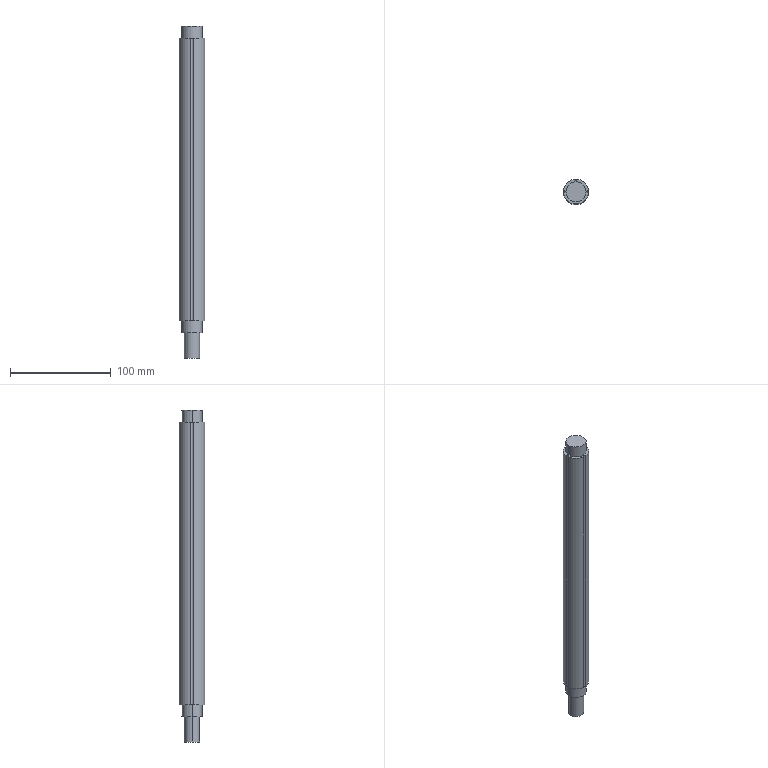Part | SolidWorks | features ICE 4, CirPattern 1, Extrusion 1 | 1 solid | 20 faces | box 24.846 x 24.846 x 329 mm | volume 147174 mm3 | cylinder 15 | plane 5 | commonest cylinder face diameters 3 x5 20 x4 25 x4 15 x2
STEP:
#1=CARTESIAN_POINT('',(11.5,0.,280.));
#2=VERTEX_POINT('',#1);
#3=CARTESIAN_POINT('',(12.423,1.385,280.));
#4=VERTEX_POINT('',#3);
#5=CARTESIAN_POINT('',(13.,0.,280.));
#6=DIRECTION('',(0.,0.,-1.));
#7=DIRECTION('',(1.,0.,0.));
#8=AXIS2_PLACEMENT_3D('',#5,#6,#7);
#9=CIRCLE('',#8,1.5);
#10=EDGE_CURVE('',#2,#4,#9,.T.);
#11=ORIENTED_EDGE('',*,*,#10,.F.);
#12=CARTESIAN_POINT('',(11.5,0.,0.));
#13=VERTEX_POINT('',#12);
#14=CARTESIAN_POINT('',(11.5,0.,284.243));
#15=DIRECTION('',(0.,0.,-1.));
#16=VECTOR('',#15,1000.);
#17=LINE('',#14,#16);
#18=EDGE_CURVE('',#2,#13,#17,.T.);
#19=ORIENTED_EDGE('',*,*,#18,.T.);
#20=CARTESIAN_POINT('',(12.423,1.385,0.));
#21=VERTEX_POINT('',#20);
#22=CARTESIAN_POINT('',(13.,0.,0.));
#23=DIRECTION('',(0.,0.,-1.));
#24=DIRECTION('',(0.,1.,0.));
#25=AXIS2_PLACEMENT_3D('',#22,#23,#24);
#26=CIRCLE('',#25,1.5);
#27=EDGE_CURVE('',#13,#21,#26,.T.);
#28=ORIENTED_EDGE('',*,*,#27,.T.);
#29=CARTESIAN_POINT('',(12.423,1.385,140.));
#30=DIRECTION('',(0.,0.,-1.));
#31=VECTOR('',#30,1000.);
#32=LINE('',#29,#31);
#33=EDGE_CURVE('',#4,#21,#32,.T.);
#34=ORIENTED_EDGE('',*,*,#33,.F.);
#35=EDGE_LOOP('',(#11,#19,#28,#34));
#36=FACE_OUTER_BOUND('',#35,.T.);
#37=CARTESIAN_POINT('',(13.,0.,284.243));
#38=DIRECTION('',(0.,0.,-1.));
#39=DIRECTION('',(-1.,0.,0.));
#40=AXIS2_PLACEMENT_3D('',#37,#38,#39);
#41=CYLINDRICAL_SURFACE('',#40,1.5);
#42=ADVANCED_FACE('',(#36),#41,.F.);
#43=CARTESIAN_POINT('',(-7.5,0.,-37.));
#44=VERTEX_POINT('',#43);
#45=CARTESIAN_POINT('',(7.5,0.,-37.));
#46=VERTEX_POINT('',#45);
#47=CARTESIAN_POINT('',(0.,0.,-37.));
#48=DIRECTION('',(0.,0.,-1.));
#49=DIRECTION('',(-1.,0.,0.));
#50=AXIS2_PLACEMENT_3D('',#47,#48,#49);
#51=CIRCLE('',#50,7.5);
#52=EDGE_CURVE('',#44,#46,#51,.T.);
#53=ORIENTED_EDGE('',*,*,#52,.F.);
#54=CARTESIAN_POINT('',(-7.5,0.,-12.));
#55=VERTEX_POINT('',#54);
#56=CARTESIAN_POINT('',(-7.5,0.,-37.));
#57=DIRECTION('',(0.,0.,1.));
#58=VECTOR('',#57,1000.);
#59=LINE('',#56,#58);
#60=EDGE_CURVE('',#44,#55,#59,.T.);
#61=ORIENTED_EDGE('',*,*,#60,.T.);
#62=CARTESIAN_POINT('',(7.5,0.,-12.));
#63=VERTEX_POINT('',#62);
#64=CARTESIAN_POINT('',(0.,0.,-12.));
#65=DIRECTION('',(0.,0.,-1.));
#66=DIRECTION('',(-1.,0.,0.));
#67=AXIS2_PLACEMENT_3D('',#64,#65,#66);
#68=CIRCLE('',#67,7.5);
#69=EDGE_CURVE('',#55,#63,#68,.T.);
#70=ORIENTED_EDGE('',*,*,#69,.T.);
#71=CARTESIAN_POINT('',(7.5,0.,-37.));
#72=DIRECTION('',(0.,0.,1.));
#73=VECTOR('',#72,1000.);
#74=LINE('',#71,#73);
#75=EDGE_CURVE('',#46,#63,#74,.T.);
#76=ORIENTED_EDGE('',*,*,#75,.F.);
#77=EDGE_LOOP('',(#53,#61,#70,#76));
#78=FACE_OUTER_BOUND('',#77,.T.);
#79=CARTESIAN_POINT('',(0.,0.,-37.));
#80=DIRECTION('',(0.,0.,1.));
#81=DIRECTION('',(1.,0.,0.));
#82=AXIS2_PLACEMENT_3D('',#79,#80,#81);
#83=CYLINDRICAL_SURFACE('',#82,7.5);
#84=ADVANCED_FACE('',(#78),#83,.T.);
#85=CARTESIAN_POINT('',(-10.,0.,-12.));
#86=VERTEX_POINT('',#85);
#87=CARTESIAN_POINT('',(10.,0.,-12.));
#88=VERTEX_POINT('',#87);
#89=CARTESIAN_POINT('',(0.,0.,-12.));
#90=DIRECTION('',(0.,0.,-1.));
#91=DIRECTION('',(-1.,0.,0.));
#92=AXIS2_PLACEMENT_3D('',#89,#90,#91);
#93=CIRCLE('',#92,10.);
#94=EDGE_CURVE('',#86,#88,#93,.T.);
#95=ORIENTED_EDGE('',*,*,#94,.F.);
#96=CARTESIAN_POINT('',(-10.,0.,0.));
#97=VERTEX_POINT('',#96);
#98=CARTESIAN_POINT('',(-10.,0.,-12.));
#99=DIRECTION('',(0.,0.,1.));
#100=VECTOR('',#99,1000.);
#101=LINE('',#98,#100);
#102=EDGE_CURVE('',#86,#97,#101,.T.);
#103=ORIENTED_EDGE('',*,*,#102,.T.);
#104=CARTESIAN_POINT('',(10.,0.,0.));
#105=VERTEX_POINT('',#104);
#106=CARTESIAN_POINT('',(0.,0.,0.));
#107=DIRECTION('',(0.,0.,-1.));
#108=DIRECTION('',(-1.,0.,0.));
#109=AXIS2_PLACEMENT_3D('',#106,#107,#108);
#110=CIRCLE('',#109,10.);
#111=EDGE_CURVE('',#97,#105,#110,.T.);
#112=ORIENTED_EDGE('',*,*,#111,.T.);
#113=CARTESIAN_POINT('',(10.,0.,-12.));
#114=DIRECTION('',(0.,0.,1.));
#115=VECTOR('',#114,1000.);
#116=LINE('',#113,#115);
#117=EDGE_CURVE('',#88,#105,#116,.T.);
#118=ORIENTED_EDGE('',*,*,#117,.F.);
#119=EDGE_LOOP('',(#95,#103,#112,#118));
#120=FACE_OUTER_BOUND('',#119,.T.);
#121=CARTESIAN_POINT('',(0.,0.,-12.));
#122=DIRECTION('',(0.,0.,1.));
#123=DIRECTION('',(1.,0.,0.));
#124=AXIS2_PLACEMENT_3D('',#121,#122,#123);
#125=CYLINDRICAL_SURFACE('',#124,10.);
#126=ADVANCED_FACE('',(#120),#125,.T.);
#127=CARTESIAN_POINT('',(10.,0.,292.));
#128=VERTEX_POINT('',#127);
#129=CARTESIAN_POINT('',(-10.,0.,292.));
#130=VERTEX_POINT('',#129);
#131=CARTESIAN_POINT('',(0.,0.,292.));
#132=DIRECTION('',(0.,0.,1.));
#133=DIRECTION('',(1.,0.,0.));
#134=AXIS2_PLACEMENT_3D('',#131,#132,#133);
#135=CIRCLE('',#134,10.);
#136=EDGE_CURVE('',#128,#130,#135,.T.);
#137=ORIENTED_EDGE('',*,*,#136,.F.);
#138=CARTESIAN_POINT('',(10.,0.,280.));
#139=VERTEX_POINT('',#138);
#140=CARTESIAN_POINT('',(10.,0.,292.));
#141=DIRECTION('',(0.,0.,-1.));
#142=VECTOR('',#141,1000.);
#143=LINE('',#140,#142);
#144=EDGE_CURVE('',#128,#139,#143,.T.);
#145=ORIENTED_EDGE('',*,*,#144,.T.);
#146=CARTESIAN_POINT('',(-10.,0.,280.));
#147=VERTEX_POINT('',#146);
#148=CARTESIAN_POINT('',(0.,0.,280.));
#149=DIRECTION('',(0.,0.,1.));
#150=DIRECTION('',(1.,0.,0.));
#151=AXIS2_PLACEMENT_3D('',#148,#149,#150);
#152=CIRCLE('',#151,10.);
#153=EDGE_CURVE('',#139,#147,#152,.T.);
#154=ORIENTED_EDGE('',*,*,#153,.T.);
#155=CARTESIAN_POINT('',(-10.,0.,292.));
#156=DIRECTION('',(0.,0.,-1.));
#157=VECTOR('',#156,1000.);
#158=LINE('',#155,#157);
#159=EDGE_CURVE('',#130,#147,#158,.T.);
#160=ORIENTED_EDGE('',*,*,#159,.F.);
#161=EDGE_LOOP('',(#137,#145,#154,#160));
#162=FACE_OUTER_BOUND('',#161,.T.);
#163=CARTESIAN_POINT('',(0.,0.,292.));
#164=DIRECTION('',(0.,0.,-1.));
#165=DIRECTION('',(-1.,0.,0.));
#166=AXIS2_PLACEMENT_3D('',#163,#164,#165);
#167=CYLINDRICAL_SURFACE('',#166,10.);
#168=ADVANCED_FACE('',(#162),#167,.T.);
#169=CARTESIAN_POINT('',(1.385,-12.423,0.));
#170=VERTEX_POINT('',#169);
#171=CARTESIAN_POINT('',(12.423,-1.385,0.));
#172=VERTEX_POINT('',#171);
#173=CARTESIAN_POINT('',(0.,0.,0.));
#174=DIRECTION('',(0.,0.,1.));
#175=DIRECTION('',(1.,0.,0.));
#176=AXIS2_PLACEMENT_3D('',#173,#174,#175);
#177=CIRCLE('',#176,12.5);
#178=EDGE_CURVE('',#170,#172,#177,.T.);
#179=ORIENTED_EDGE('',*,*,#178,.T.);
#180=CARTESIAN_POINT('',(12.423,-1.385,280.));
#181=VERTEX_POINT('',#180);
#182=CARTESIAN_POINT('',(12.423,-1.385,140.));
#183=DIRECTION('',(0.,0.,1.));
#184=VECTOR('',#183,1000.);
#185=LINE('',#182,#184);
#186=EDGE_CURVE('',#172,#181,#185,.T.);
#187=ORIENTED_EDGE('',*,*,#186,.T.);
#188=CARTESIAN_POINT('',(1.385,-12.423,280.));
#189=VERTEX_POINT('',#188);
#190=CARTESIAN_POINT('',(0.,0.,280.));
#191=DIRECTION('',(0.,0.,1.));
#192=DIRECTION('',(1.,0.,0.));
#193=AXIS2_PLACEMENT_3D('',#190,#191,#192);
#194=CIRCLE('',#193,12.5);
#195=EDGE_CURVE('',#189,#181,#194,.T.);
#196=ORIENTED_EDGE('',*,*,#195,.F.);
#197=CARTESIAN_POINT('',(1.385,-12.423,140.));
#198=DIRECTION('',(0.,0.,-1.));
#199=VECTOR('',#198,1000.);
#200=LINE('',#197,#199);
#201=EDGE_CURVE('',#189,#170,#200,.T.);
#202=ORIENTED_EDGE('',*,*,#201,.T.);
#203=EDGE_LOOP('',(#179,#187,#196,#202));
#204=FACE_OUTER_BOUND('',#203,.T.);
#205=CARTESIAN_POINT('',(0.,0.,280.));
#206=DIRECTION('',(0.,0.,-1.));
#207=DIRECTION('',(-1.,0.,0.));
#208=AXIS2_PLACEMENT_3D('',#205,#206,#207);
#209=CYLINDRICAL_SURFACE('',#208,12.5);
#210=ADVANCED_FACE('',(#204),#209,.T.);
#211=CARTESIAN_POINT('',(-12.423,-1.385,0.));
#212=VERTEX_POINT('',#211);
#213=CARTESIAN_POINT('',(-1.385,-12.423,0.));
#214=VERTEX_POINT('',#213);
#215=CARTESIAN_POINT('',(0.,0.,0.));
#216=DIRECTION('',(0.,0.,1.));
#217=DIRECTION('',(1.,0.,0.));
#218=AXIS2_PLACEMENT_3D('',#215,#216,#217);
#219=CIRCLE('',#218,12.5);
#220=EDGE_CURVE('',#212,#214,#219,.T.);
#221=ORIENTED_EDGE('',*,*,#220,.T.);
#222=CARTESIAN_POINT('',(-1.385,-12.423,280.));
#223=VERTEX_POINT('',#222);
#224=CARTESIAN_POINT('',(-1.385,-12.423,140.));
#225=DIRECTION('',(0.,0.,1.));
#226=VECTOR('',#225,1000.);
#227=LINE('',#224,#226);
#228=EDGE_CURVE('',#214,#223,#227,.T.);
#229=ORIENTED_EDGE('',*,*,#228,.T.);
#230=CARTESIAN_POINT('',(-12.423,-1.385,280.));
#231=VERTEX_POINT('',#230);
#232=CARTESIAN_POINT('',(0.,0.,280.));
#233=DIRECTION('',(0.,0.,1.));
#234=DIRECTION('',(1.,0.,0.));
#235=AXIS2_PLACEMENT_3D('',#232,#233,#234);
#236=CIRCLE('',#235,12.5);
#237=EDGE_CURVE('',#231,#223,#236,.T.);
#238=ORIENTED_EDGE('',*,*,#237,.F.);
#239=CARTESIAN_POINT('',(-12.423,-1.385,140.));
#240=DIRECTION('',(0.,0.,-1.));
#241=VECTOR('',#240,1000.);
#242=LINE('',#239,#241);
#243=EDGE_CURVE('',#231,#212,#242,.T.);
#244=ORIENTED_EDGE('',*,*,#243,.T.);
#245=EDGE_LOOP('',(#221,#229,#238,#244));
#246=FACE_OUTER_BOUND('',#245,.T.);
#247=CARTESIAN_POINT('',(0.,0.,280.));
#248=DIRECTION('',(0.,0.,-1.));
#249=DIRECTION('',(-1.,0.,0.));
#250=AXIS2_PLACEMENT_3D('',#247,#248,#249);
#251=CYLINDRICAL_SURFACE('',#250,12.5);
#252=ADVANCED_FACE('',(#246),#251,.T.);
#253=CARTESIAN_POINT('',(-1.385,12.423,0.));
#254=VERTEX_POINT('',#253);
#255=CARTESIAN_POINT('',(-12.423,1.385,0.));
#256=VERTEX_POINT('',#255);
#257=CARTESIAN_POINT('',(0.,0.,0.));
#258=DIRECTION('',(0.,0.,1.));
#259=DIRECTION('',(1.,0.,0.));
#260=AXIS2_PLACEMENT_3D('',#257,#258,#259);
#261=CIRCLE('',#260,12.5);
#262=EDGE_CURVE('',#254,#256,#261,.T.);
#263=ORIENTED_EDGE('',*,*,#262,.T.);
#264=CARTESIAN_POINT('',(-12.423,1.385,280.));
#265=VERTEX_POINT('',#264);
#266=CARTESIAN_POINT('',(-12.423,1.385,140.));
#267=DIRECTION('',(0.,0.,1.));
#268=VECTOR('',#267,1000.);
#269=LINE('',#266,#268);
#270=EDGE_CURVE('',#256,#265,#269,.T.);
#271=ORIENTED_EDGE('',*,*,#270,.T.);
#272=CARTESIAN_POINT('',(-1.385,12.423,280.));
#273=VERTEX_POINT('',#272);
#274=CARTESIAN_POINT('',(0.,0.,280.));
#275=DIRECTION('',(0.,0.,1.));
#276=DIRECTION('',(1.,0.,0.));
#277=AXIS2_PLACEMENT_3D('',#274,#275,#276);
#278=CIRCLE('',#277,12.5);
#279=EDGE_CURVE('',#273,#265,#278,.T.);
#280=ORIENTED_EDGE('',*,*,#279,.F.);
#281=CARTESIAN_POINT('',(-1.385,12.423,140.));
#282=DIRECTION('',(0.,0.,-1.));
#283=VECTOR('',#282,1000.);
#284=LINE('',#281,#283);
#285=EDGE_CURVE('',#273,#254,#284,.T.);
#286=ORIENTED_EDGE('',*,*,#285,.T.);
#287=EDGE_LOOP('',(#263,#271,#280,#286));
#288=FACE_OUTER_BOUND('',#287,.T.);
#289=CARTESIAN_POINT('',(0.,0.,280.));
#290=DIRECTION('',(0.,0.,-1.));
#291=DIRECTION('',(-1.,0.,0.));
#292=AXIS2_PLACEMENT_3D('',#289,#290,#291);
#293=CYLINDRICAL_SURFACE('',#292,12.5);
#294=ADVANCED_FACE('',(#288),#293,.T.);
#295=CARTESIAN_POINT('',(1.385,12.423,280.));
#296=VERTEX_POINT('',#295);
#297=CARTESIAN_POINT('',(0.,0.,280.));
#298=DIRECTION('',(0.,0.,1.));
#299=DIRECTION('',(1.,0.,0.));
#300=AXIS2_PLACEMENT_3D('',#297,#298,#299);
#301=CIRCLE('',#300,12.5);
#302=EDGE_CURVE('',#4,#296,#301,.T.);
#303=ORIENTED_EDGE('',*,*,#302,.F.);
#304=ORIENTED_EDGE('',*,*,#33,.T.);
#305=CARTESIAN_POINT('',(1.385,12.423,0.));
#306=VERTEX_POINT('',#305);
#307=CARTESIAN_POINT('',(0.,0.,0.));
#308=DIRECTION('',(0.,0.,1.));
#309=DIRECTION('',(1.,0.,0.));
#310=AXIS2_PLACEMENT_3D('',#307,#308,#309);
#311=CIRCLE('',#310,12.5);
#312=EDGE_CURVE('',#21,#306,#311,.T.);
#313=ORIENTED_EDGE('',*,*,#312,.T.);
#314=CARTESIAN_POINT('',(1.385,12.423,140.));
#315=DIRECTION('',(0.,0.,1.));
#316=VECTOR('',#315,1000.);
#317=LINE('',#314,#316);
#318=EDGE_CURVE('',#306,#296,#317,.T.);
#319=ORIENTED_EDGE('',*,*,#318,.T.);
#320=EDGE_LOOP('',(#303,#304,#313,#319));
#321=FACE_OUTER_BOUND('',#320,.T.);
#322=CARTESIAN_POINT('',(0.,0.,280.));
#323=DIRECTION('',(0.,0.,-1.));
#324=DIRECTION('',(-1.,0.,0.));
#325=AXIS2_PLACEMENT_3D('',#322,#323,#324);
#326=CYLINDRICAL_SURFACE('',#325,12.5);
#327=ADVANCED_FACE('',(#321),#326,.T.);
#328=CARTESIAN_POINT('',(13.,0.,280.));
#329=DIRECTION('',(0.,0.,-1.));
#330=DIRECTION('',(1.,0.,0.));
#331=AXIS2_PLACEMENT_3D('',#328,#329,#330);
#332=CIRCLE('',#331,1.5);
#333=EDGE_CURVE('',#181,#2,#332,.T.);
#334=ORIENTED_EDGE('',*,*,#333,.T.);
#335=ORIENTED_EDGE('',*,*,#10,.T.);
#336=ORIENTED_EDGE('',*,*,#302,.T.);
#337=CARTESIAN_POINT('',(0.,13.,280.));
#338=DIRECTION('',(0.,0.,-1.));
#339=DIRECTION('',(1.,0.,0.));
#340=AXIS2_PLACEMENT_3D('',#337,#338,#339);
#341=CIRCLE('',#340,1.5);
#342=EDGE_CURVE('',#296,#273,#341,.T.);
#343=ORIENTED_EDGE('',*,*,#342,.T.);
#344=ORIENTED_EDGE('',*,*,#279,.T.);
#345=CARTESIAN_POINT('',(-13.,0.,280.));
#346=DIRECTION('',(0.,0.,-1.));
#347=DIRECTION('',(1.,0.,0.));
#348=AXIS2_PLACEMENT_3D('',#345,#346,#347);
#349=CIRCLE('',#348,1.5);
#350=EDGE_CURVE('',#265,#231,#349,.T.);
#351=ORIENTED_EDGE('',*,*,#350,.T.);
#352=ORIENTED_EDGE('',*,*,#237,.T.);
#353=CARTESIAN_POINT('',(0.,-13.,280.));
#354=DIRECTION('',(0.,0.,-1.));
#355=DIRECTION('',(1.,0.,0.));
#356=AXIS2_PLACEMENT_3D('',#353,#354,#355);
#357=CIRCLE('',#356,1.5);
#358=EDGE_CURVE('',#223,#189,#357,.T.);
#359=ORIENTED_EDGE('',*,*,#358,.T.);
#360=ORIENTED_EDGE('',*,*,#195,.T.);
#361=EDGE_LOOP('',(#334,#335,#336,#343,#344,#351,#352,#359,#360));
#362=FACE_OUTER_BOUND('',#361,.T.);
#363=CARTESIAN_POINT('',(0.,0.,280.));
#364=DIRECTION('',(0.,0.,1.));
#365=DIRECTION('',(1.,0.,0.));
#366=AXIS2_PLACEMENT_3D('',#363,#364,#365);
#367=CIRCLE('',#366,10.);
#368=EDGE_CURVE('',#147,#139,#367,.T.);
#369=ORIENTED_EDGE('',*,*,#368,.F.);
#370=ORIENTED_EDGE('',*,*,#153,.F.);
#371=EDGE_LOOP('',(#369,#370));
#372=FACE_BOUND('',#371,.T.);
#373=CARTESIAN_POINT('',(0.,0.,280.));
#374=DIRECTION('',(0.,0.,1.));
#375=DIRECTION('',(1.,0.,0.));
#376=AXIS2_PLACEMENT_3D('',#373,#374,#375);
#377=PLANE('',#376);
#378=ADVANCED_FACE('',(#362,#372),#377,.T.);
#379=CARTESIAN_POINT('',(0.,0.,0.));
#380=DIRECTION('',(0.,0.,-1.));
#381=DIRECTION('',(-1.,0.,0.));
#382=AXIS2_PLACEMENT_3D('',#379,#380,#381);
#383=CIRCLE('',#382,10.);
#384=EDGE_CURVE('',#105,#97,#383,.T.);
#385=ORIENTED_EDGE('',*,*,#384,.F.);
#386=ORIENTED_EDGE('',*,*,#111,.F.);
#387=EDGE_LOOP('',(#385,#386));
#388=FACE_BOUND('',#387,.T.);
#389=ORIENTED_EDGE('',*,*,#312,.F.);
#390=ORIENTED_EDGE('',*,*,#27,.F.);
#391=CARTESIAN_POINT('',(13.,0.,0.));
#392=DIRECTION('',(0.,0.,-1.));
#393=DIRECTION('',(0.,1.,0.));
#394=AXIS2_PLACEMENT_3D('',#391,#392,#393);
#395=CIRCLE('',#394,1.5);
#396=EDGE_CURVE('',#172,#13,#395,.T.);
#397=ORIENTED_EDGE('',*,*,#396,.F.);
#398=ORIENTED_EDGE('',*,*,#178,.F.);
#399=CARTESIAN_POINT('',(0.,-13.,0.));
#400=DIRECTION('',(0.,0.,-1.));
#401=DIRECTION('',(1.,0.,0.));
#402=AXIS2_PLACEMENT_3D('',#399,#400,#401);
#403=CIRCLE('',#402,1.5);
#404=EDGE_CURVE('',#214,#170,#403,.T.);
#405=ORIENTED_EDGE('',*,*,#404,.F.);
#406=ORIENTED_EDGE('',*,*,#220,.F.);
#407=CARTESIAN_POINT('',(-13.,0.,0.));
#408=DIRECTION('',(0.,0.,-1.));
#409=DIRECTION('',(0.,-1.,0.));
#410=AXIS2_PLACEMENT_3D('',#407,#408,#409);
#411=CIRCLE('',#410,1.5);
#412=EDGE_CURVE('',#256,#212,#411,.T.);
#413=ORIENTED_EDGE('',*,*,#412,.F.);
#414=ORIENTED_EDGE('',*,*,#262,.F.);
#415=CARTESIAN_POINT('',(0.,13.,0.));
#416=DIRECTION('',(0.,0.,-1.));
#417=DIRECTION('',(-1.,0.,0.));
#418=AXIS2_PLACEMENT_3D('',#415,#416,#417);
#419=CIRCLE('',#418,1.5);
#420=EDGE_CURVE('',#306,#254,#419,.T.);
#421=ORIENTED_EDGE('',*,*,#420,.F.);
#422=EDGE_LOOP('',(#389,#390,#397,#398,#405,#406,#413,#414,#421));
#423=FACE_OUTER_BOUND('',#422,.T.);
#424=CARTESIAN_POINT('',(0.,0.,0.));
#425=DIRECTION('',(0.,0.,1.));
#426=DIRECTION('',(1.,0.,0.));
#427=AXIS2_PLACEMENT_3D('',#424,#425,#426);
#428=PLANE('',#427);
#429=ADVANCED_FACE('',(#388,#423),#428,.F.);
#430=ORIENTED_EDGE('',*,*,#144,.F.);
#431=CARTESIAN_POINT('',(0.,0.,292.));
#432=DIRECTION('',(0.,0.,1.));
#433=DIRECTION('',(1.,0.,0.));
#434=AXIS2_PLACEMENT_3D('',#431,#432,#433);
#435=CIRCLE('',#434,10.);
#436=EDGE_CURVE('',#130,#128,#435,.T.);
#437=ORIENTED_EDGE('',*,*,#436,.F.);
#438=ORIENTED_EDGE('',*,*,#159,.T.);
#439=ORIENTED_EDGE('',*,*,#368,.T.);
#440=EDGE_LOOP('',(#430,#437,#438,#439));
#441=FACE_OUTER_BOUND('',#440,.T.);
#442=CARTESIAN_POINT('',(0.,0.,292.));
#443=DIRECTION('',(0.,0.,-1.));
#444=DIRECTION('',(-1.,0.,0.));
#445=AXIS2_PLACEMENT_3D('',#442,#443,#444);
#446=CYLINDRICAL_SURFACE('',#445,10.);
#447=ADVANCED_FACE('',(#441),#446,.T.);
#448=ORIENTED_EDGE('',*,*,#436,.T.);
#449=ORIENTED_EDGE('',*,*,#136,.T.);
#450=EDGE_LOOP('',(#448,#449));
#451=FACE_OUTER_BOUND('',#450,.T.);
#452=CARTESIAN_POINT('',(0.,0.,292.));
#453=DIRECTION('',(0.,0.,1.));
#454=DIRECTION('',(1.,0.,0.));
#455=AXIS2_PLACEMENT_3D('',#452,#453,#454);
#456=PLANE('',#455);
#457=ADVANCED_FACE('',(#451),#456,.T.);
#458=ORIENTED_EDGE('',*,*,#102,.F.);
#459=CARTESIAN_POINT('',(0.,0.,-12.));
#460=DIRECTION('',(0.,0.,-1.));
#461=DIRECTION('',(-1.,0.,0.));
#462=AXIS2_PLACEMENT_3D('',#459,#460,#461);
#463=CIRCLE('',#462,10.);
#464=EDGE_CURVE('',#88,#86,#463,.T.);
#465=ORIENTED_EDGE('',*,*,#464,.F.);
#466=ORIENTED_EDGE('',*,*,#117,.T.);
#467=ORIENTED_EDGE('',*,*,#384,.T.);
#468=EDGE_LOOP('',(#458,#465,#466,#467));
#469=FACE_OUTER_BOUND('',#468,.T.);
#470=CARTESIAN_POINT('',(0.,0.,-12.));
#471=DIRECTION('',(0.,0.,1.));
#472=DIRECTION('',(1.,0.,0.));
#473=AXIS2_PLACEMENT_3D('',#470,#471,#472);
#474=CYLINDRICAL_SURFACE('',#473,10.);
#475=ADVANCED_FACE('',(#469),#474,.T.);
#476=CARTESIAN_POINT('',(0.,0.,-12.));
#477=DIRECTION('',(0.,0.,-1.));
#478=DIRECTION('',(-1.,0.,0.));
#479=AXIS2_PLACEMENT_3D('',#476,#477,#478);
#480=CIRCLE('',#479,7.5);
#481=EDGE_CURVE('',#63,#55,#480,.T.);
#482=ORIENTED_EDGE('',*,*,#481,.F.);
#483=ORIENTED_EDGE('',*,*,#69,.F.);
#484=EDGE_LOOP('',(#482,#483));
#485=FACE_BOUND('',#484,.T.);
#486=ORIENTED_EDGE('',*,*,#464,.T.);
#487=ORIENTED_EDGE('',*,*,#94,.T.);
#488=EDGE_LOOP('',(#486,#487));
#489=FACE_OUTER_BOUND('',#488,.T.);
#490=CARTESIAN_POINT('',(0.,0.,-12.));
#491=DIRECTION('',(0.,0.,-1.));
#492=DIRECTION('',(-1.,0.,0.));
#493=AXIS2_PLACEMENT_3D('',#490,#491,#492);
#494=PLANE('',#493);
#495=ADVANCED_FACE('',(#485,#489),#494,.T.);
#496=ORIENTED_EDGE('',*,*,#60,.F.);
#497=CARTESIAN_POINT('',(0.,0.,-37.));
#498=DIRECTION('',(0.,0.,-1.));
#499=DIRECTION('',(-1.,0.,0.));
#500=AXIS2_PLACEMENT_3D('',#497,#498,#499);
#501=CIRCLE('',#500,7.5);
#502=EDGE_CURVE('',#46,#44,#501,.T.);
#503=ORIENTED_EDGE('',*,*,#502,.F.);
#504=ORIENTED_EDGE('',*,*,#75,.T.);
#505=ORIENTED_EDGE('',*,*,#481,.T.);
#506=EDGE_LOOP('',(#496,#503,#504,#505));
#507=FACE_OUTER_BOUND('',#506,.T.);
#508=CARTESIAN_POINT('',(0.,0.,-37.));
#509=DIRECTION('',(0.,0.,1.));
#510=DIRECTION('',(1.,0.,0.));
#511=AXIS2_PLACEMENT_3D('',#508,#509,#510);
#512=CYLINDRICAL_SURFACE('',#511,7.5);
#513=ADVANCED_FACE('',(#507),#512,.T.);
#514=ORIENTED_EDGE('',*,*,#502,.T.);
#515=ORIENTED_EDGE('',*,*,#52,.T.);
#516=EDGE_LOOP('',(#514,#515));
#517=FACE_OUTER_BOUND('',#516,.T.);
#518=CARTESIAN_POINT('',(0.,0.,-37.));
#519=DIRECTION('',(0.,0.,-1.));
#520=DIRECTION('',(-1.,0.,0.));
#521=AXIS2_PLACEMENT_3D('',#518,#519,#520);
#522=PLANE('',#521);
#523=ADVANCED_FACE('',(#517),#522,.T.);
#524=ORIENTED_EDGE('',*,*,#420,.T.);
#525=ORIENTED_EDGE('',*,*,#285,.F.);
#526=ORIENTED_EDGE('',*,*,#342,.F.);
#527=ORIENTED_EDGE('',*,*,#318,.F.);
#528=EDGE_LOOP('',(#524,#525,#526,#527));
#529=FACE_OUTER_BOUND('',#528,.T.);
#530=CARTESIAN_POINT('',(0.,13.,284.243));
#531=DIRECTION('',(0.,0.,-1.));
#532=DIRECTION('',(-1.,0.,0.));
#533=AXIS2_PLACEMENT_3D('',#530,#531,#532);
#534=CYLINDRICAL_SURFACE('',#533,1.5);
#535=ADVANCED_FACE('',(#529),#534,.F.);
#536=ORIENTED_EDGE('',*,*,#412,.T.);
#537=ORIENTED_EDGE('',*,*,#243,.F.);
#538=ORIENTED_EDGE('',*,*,#350,.F.);
#539=ORIENTED_EDGE('',*,*,#270,.F.);
#540=EDGE_LOOP('',(#536,#537,#538,#539));
#541=FACE_OUTER_BOUND('',#540,.T.);
#542=CARTESIAN_POINT('',(-13.,0.,284.243));
#543=DIRECTION('',(0.,0.,-1.));
#544=DIRECTION('',(-1.,0.,0.));
#545=AXIS2_PLACEMENT_3D('',#542,#543,#544);
#546=CYLINDRICAL_SURFACE('',#545,1.5);
#547=ADVANCED_FACE('',(#541),#546,.F.);
#548=ORIENTED_EDGE('',*,*,#404,.T.);
#549=ORIENTED_EDGE('',*,*,#201,.F.);
#550=ORIENTED_EDGE('',*,*,#358,.F.);
#551=ORIENTED_EDGE('',*,*,#228,.F.);
#552=EDGE_LOOP('',(#548,#549,#550,#551));
#553=FACE_OUTER_BOUND('',#552,.T.);
#554=CARTESIAN_POINT('',(0.,-13.,284.243));
#555=DIRECTION('',(0.,0.,-1.));
#556=DIRECTION('',(-1.,0.,0.));
#557=AXIS2_PLACEMENT_3D('',#554,#555,#556);
#558=CYLINDRICAL_SURFACE('',#557,1.5);
#559=ADVANCED_FACE('',(#553),#558,.F.);
#560=ORIENTED_EDGE('',*,*,#18,.F.);
#561=ORIENTED_EDGE('',*,*,#333,.F.);
#562=ORIENTED_EDGE('',*,*,#186,.F.);
#563=ORIENTED_EDGE('',*,*,#396,.T.);
#564=EDGE_LOOP('',(#560,#561,#562,#563));
#565=FACE_OUTER_BOUND('',#564,.T.);
#566=CARTESIAN_POINT('',(13.,0.,284.243));
#567=DIRECTION('',(0.,0.,-1.));
#568=DIRECTION('',(-1.,0.,0.));
#569=AXIS2_PLACEMENT_3D('',#566,#567,#568);
#570=CYLINDRICAL_SURFACE('',#569,1.5);
#571=ADVANCED_FACE('',(#565),#570,.F.);
#572=CLOSED_SHELL('',(#42,#84,#126,#168,#210,#252,#294,#327,#378,#429,#447,#457,#475,#495,#513,#523,#535,#547,#559,#571));
#573=MANIFOLD_SOLID_BREP('',#572);
#574=CARTESIAN_POINT('',(0.,0.,0.));
#575=DIRECTION('',(0.,0.,1.));
#576=DIRECTION('',(1.,0.,0.));
#577=AXIS2_PLACEMENT_3D('',#574,#575,#576);
#578=(LENGTH_UNIT()NAMED_UNIT(*)SI_UNIT(.MILLI.,.METRE.));
#579=UNCERTAINTY_MEASURE_WITH_UNIT(LENGTH_MEASURE(0.00001),#578,'','');
#580=(NAMED_UNIT(*)PLANE_ANGLE_UNIT()SI_UNIT($,.RADIAN.));
#581=(NAMED_UNIT(*)SI_UNIT($,.STERADIAN.)SOLID_ANGLE_UNIT());
#582=(GEOMETRIC_REPRESENTATION_CONTEXT(3)GLOBAL_UNCERTAINTY_ASSIGNED_CONTEXT((#579))GLOBAL_UNIT_ASSIGNED_CONTEXT((#578,#580,#581))REPRESENTATION_CONTEXT('',''));
#583=ADVANCED_BREP_SHAPE_REPRESENTATION('',(#573,#577),#582);